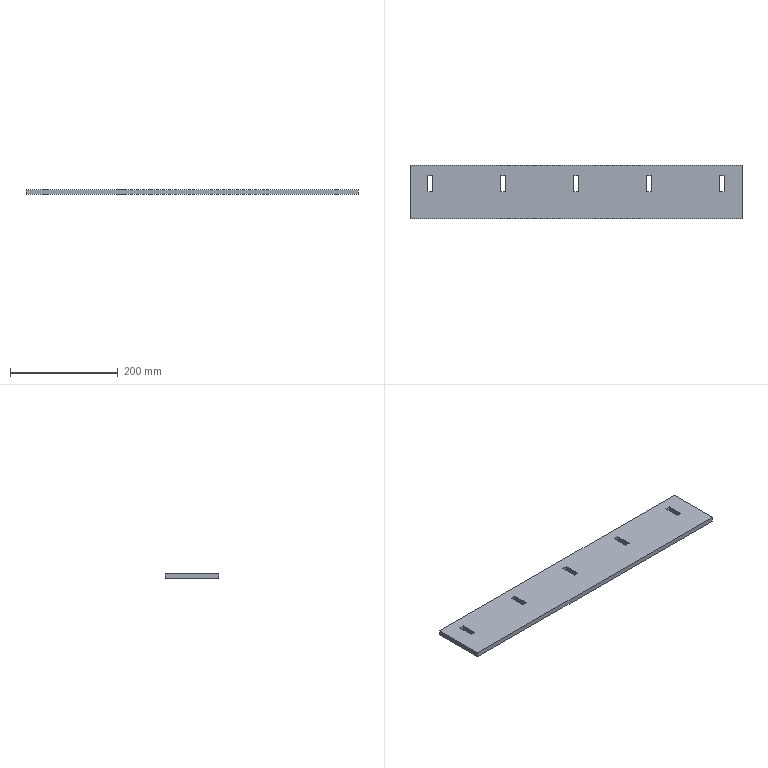Part | SolidWorks | features FlatPattern 1, SMBaseFlange 1, SheetMetal 1 | 1 solid | 26 faces | box 615 x 100 x 9 mm | volume 541350 mm3 | plane 26
STEP:
#1=CARTESIAN_POINT('',(269.54,-128.583,9.));
#2=VERTEX_POINT('',#1);
#3=CARTESIAN_POINT('',(269.54,-28.583,9.));
#4=VERTEX_POINT('',#3);
#5=CARTESIAN_POINT('',(269.54,-128.583,9.));
#6=DIRECTION('',(0.,1.,0.));
#7=VECTOR('',#6,1000.);
#8=LINE('',#5,#7);
#9=EDGE_CURVE('',#2,#4,#8,.T.);
#10=ORIENTED_EDGE('',*,*,#9,.T.);
#11=CARTESIAN_POINT('',(-345.46,-28.583,9.));
#12=VERTEX_POINT('',#11);
#13=CARTESIAN_POINT('',(269.54,-28.583,9.));
#14=DIRECTION('',(-1.,0.,0.));
#15=VECTOR('',#14,1000.);
#16=LINE('',#13,#15);
#17=EDGE_CURVE('',#4,#12,#16,.T.);
#18=ORIENTED_EDGE('',*,*,#17,.T.);
#19=CARTESIAN_POINT('',(-345.46,-128.583,9.));
#20=VERTEX_POINT('',#19);
#21=CARTESIAN_POINT('',(-345.46,-128.583,9.));
#22=DIRECTION('',(0.,-1.,0.));
#23=VECTOR('',#22,1000.);
#24=LINE('',#21,#23);
#25=EDGE_CURVE('',#12,#20,#24,.T.);
#26=ORIENTED_EDGE('',*,*,#25,.T.);
#27=CARTESIAN_POINT('',(269.54,-128.583,9.));
#28=DIRECTION('',(1.,0.,0.));
#29=VECTOR('',#28,1000.);
#30=LINE('',#27,#29);
#31=EDGE_CURVE('',#20,#2,#30,.T.);
#32=ORIENTED_EDGE('',*,*,#31,.T.);
#33=EDGE_LOOP('',(#10,#18,#26,#32));
#34=FACE_OUTER_BOUND('',#33,.T.);
#35=CARTESIAN_POINT('',(236.54,-48.583,9.));
#36=VERTEX_POINT('',#35);
#37=CARTESIAN_POINT('',(227.54,-48.583,9.));
#38=VERTEX_POINT('',#37);
#39=CARTESIAN_POINT('',(236.54,-48.583,9.));
#40=DIRECTION('',(-1.,0.,0.));
#41=VECTOR('',#40,1000.);
#42=LINE('',#39,#41);
#43=EDGE_CURVE('',#36,#38,#42,.T.);
#44=ORIENTED_EDGE('',*,*,#43,.F.);
#45=CARTESIAN_POINT('',(236.54,-78.583,9.));
#46=VERTEX_POINT('',#45);
#47=CARTESIAN_POINT('',(236.54,-48.583,9.));
#48=DIRECTION('',(0.,1.,0.));
#49=VECTOR('',#48,1000.);
#50=LINE('',#47,#49);
#51=EDGE_CURVE('',#46,#36,#50,.T.);
#52=ORIENTED_EDGE('',*,*,#51,.F.);
#53=CARTESIAN_POINT('',(227.54,-78.583,9.));
#54=VERTEX_POINT('',#53);
#55=CARTESIAN_POINT('',(236.54,-78.583,9.));
#56=DIRECTION('',(1.,0.,0.));
#57=VECTOR('',#56,1000.);
#58=LINE('',#55,#57);
#59=EDGE_CURVE('',#54,#46,#58,.T.);
#60=ORIENTED_EDGE('',*,*,#59,.F.);
#61=CARTESIAN_POINT('',(227.54,-48.583,9.));
#62=DIRECTION('',(0.,-1.,0.));
#63=VECTOR('',#62,1000.);
#64=LINE('',#61,#63);
#65=EDGE_CURVE('',#38,#54,#64,.T.);
#66=ORIENTED_EDGE('',*,*,#65,.F.);
#67=EDGE_LOOP('',(#44,#52,#60,#66));
#68=FACE_BOUND('',#67,.T.);
#69=CARTESIAN_POINT('',(92.54,-78.583,9.));
#70=VERTEX_POINT('',#69);
#71=CARTESIAN_POINT('',(101.54,-78.583,9.));
#72=VERTEX_POINT('',#71);
#73=CARTESIAN_POINT('',(92.54,-78.583,9.));
#74=DIRECTION('',(1.,0.,0.));
#75=VECTOR('',#74,1000.);
#76=LINE('',#73,#75);
#77=EDGE_CURVE('',#70,#72,#76,.T.);
#78=ORIENTED_EDGE('',*,*,#77,.F.);
#79=CARTESIAN_POINT('',(92.54,-48.583,9.));
#80=VERTEX_POINT('',#79);
#81=CARTESIAN_POINT('',(92.54,-48.583,9.));
#82=DIRECTION('',(0.,-1.,0.));
#83=VECTOR('',#82,1000.);
#84=LINE('',#81,#83);
#85=EDGE_CURVE('',#80,#70,#84,.T.);
#86=ORIENTED_EDGE('',*,*,#85,.F.);
#87=CARTESIAN_POINT('',(101.54,-48.583,9.));
#88=VERTEX_POINT('',#87);
#89=CARTESIAN_POINT('',(92.54,-48.583,9.));
#90=DIRECTION('',(-1.,0.,0.));
#91=VECTOR('',#90,1000.);
#92=LINE('',#89,#91);
#93=EDGE_CURVE('',#88,#80,#92,.T.);
#94=ORIENTED_EDGE('',*,*,#93,.F.);
#95=CARTESIAN_POINT('',(101.54,-48.583,9.));
#96=DIRECTION('',(0.,1.,0.));
#97=VECTOR('',#96,1000.);
#98=LINE('',#95,#97);
#99=EDGE_CURVE('',#72,#88,#98,.T.);
#100=ORIENTED_EDGE('',*,*,#99,.F.);
#101=EDGE_LOOP('',(#78,#86,#94,#100));
#102=FACE_BOUND('',#101,.T.);
#103=CARTESIAN_POINT('',(-42.46,-78.583,9.));
#104=VERTEX_POINT('',#103);
#105=CARTESIAN_POINT('',(-33.46,-78.583,9.));
#106=VERTEX_POINT('',#105);
#107=CARTESIAN_POINT('',(-42.46,-78.583,9.));
#108=DIRECTION('',(1.,0.,0.));
#109=VECTOR('',#108,1000.);
#110=LINE('',#107,#109);
#111=EDGE_CURVE('',#104,#106,#110,.T.);
#112=ORIENTED_EDGE('',*,*,#111,.F.);
#113=CARTESIAN_POINT('',(-42.46,-48.583,9.));
#114=VERTEX_POINT('',#113);
#115=CARTESIAN_POINT('',(-42.46,-48.583,9.));
#116=DIRECTION('',(0.,-1.,0.));
#117=VECTOR('',#116,1000.);
#118=LINE('',#115,#117);
#119=EDGE_CURVE('',#114,#104,#118,.T.);
#120=ORIENTED_EDGE('',*,*,#119,.F.);
#121=CARTESIAN_POINT('',(-33.46,-48.583,9.));
#122=VERTEX_POINT('',#121);
#123=CARTESIAN_POINT('',(-42.46,-48.583,9.));
#124=DIRECTION('',(-1.,0.,0.));
#125=VECTOR('',#124,1000.);
#126=LINE('',#123,#125);
#127=EDGE_CURVE('',#122,#114,#126,.T.);
#128=ORIENTED_EDGE('',*,*,#127,.F.);
#129=CARTESIAN_POINT('',(-33.46,-48.583,9.));
#130=DIRECTION('',(0.,1.,0.));
#131=VECTOR('',#130,1000.);
#132=LINE('',#129,#131);
#133=EDGE_CURVE('',#106,#122,#132,.T.);
#134=ORIENTED_EDGE('',*,*,#133,.F.);
#135=EDGE_LOOP('',(#112,#120,#128,#134));
#136=FACE_BOUND('',#135,.T.);
#137=CARTESIAN_POINT('',(-177.46,-78.583,9.));
#138=VERTEX_POINT('',#137);
#139=CARTESIAN_POINT('',(-168.46,-78.583,9.));
#140=VERTEX_POINT('',#139);
#141=CARTESIAN_POINT('',(-177.46,-78.583,9.));
#142=DIRECTION('',(1.,0.,0.));
#143=VECTOR('',#142,1000.);
#144=LINE('',#141,#143);
#145=EDGE_CURVE('',#138,#140,#144,.T.);
#146=ORIENTED_EDGE('',*,*,#145,.F.);
#147=CARTESIAN_POINT('',(-177.46,-48.583,9.));
#148=VERTEX_POINT('',#147);
#149=CARTESIAN_POINT('',(-177.46,-48.583,9.));
#150=DIRECTION('',(0.,-1.,0.));
#151=VECTOR('',#150,1000.);
#152=LINE('',#149,#151);
#153=EDGE_CURVE('',#148,#138,#152,.T.);
#154=ORIENTED_EDGE('',*,*,#153,.F.);
#155=CARTESIAN_POINT('',(-168.46,-48.583,9.));
#156=VERTEX_POINT('',#155);
#157=CARTESIAN_POINT('',(-177.46,-48.583,9.));
#158=DIRECTION('',(-1.,0.,0.));
#159=VECTOR('',#158,1000.);
#160=LINE('',#157,#159);
#161=EDGE_CURVE('',#156,#148,#160,.T.);
#162=ORIENTED_EDGE('',*,*,#161,.F.);
#163=CARTESIAN_POINT('',(-168.46,-48.583,9.));
#164=DIRECTION('',(0.,1.,0.));
#165=VECTOR('',#164,1000.);
#166=LINE('',#163,#165);
#167=EDGE_CURVE('',#140,#156,#166,.T.);
#168=ORIENTED_EDGE('',*,*,#167,.F.);
#169=EDGE_LOOP('',(#146,#154,#162,#168));
#170=FACE_BOUND('',#169,.T.);
#171=CARTESIAN_POINT('',(-312.46,-78.583,9.));
#172=VERTEX_POINT('',#171);
#173=CARTESIAN_POINT('',(-303.46,-78.583,9.));
#174=VERTEX_POINT('',#173);
#175=CARTESIAN_POINT('',(-312.46,-78.583,9.));
#176=DIRECTION('',(1.,0.,0.));
#177=VECTOR('',#176,1000.);
#178=LINE('',#175,#177);
#179=EDGE_CURVE('',#172,#174,#178,.T.);
#180=ORIENTED_EDGE('',*,*,#179,.F.);
#181=CARTESIAN_POINT('',(-312.46,-48.583,9.));
#182=VERTEX_POINT('',#181);
#183=CARTESIAN_POINT('',(-312.46,-48.583,9.));
#184=DIRECTION('',(0.,-1.,0.));
#185=VECTOR('',#184,1000.);
#186=LINE('',#183,#185);
#187=EDGE_CURVE('',#182,#172,#186,.T.);
#188=ORIENTED_EDGE('',*,*,#187,.F.);
#189=CARTESIAN_POINT('',(-303.46,-48.583,9.));
#190=VERTEX_POINT('',#189);
#191=CARTESIAN_POINT('',(-312.46,-48.583,9.));
#192=DIRECTION('',(-1.,0.,0.));
#193=VECTOR('',#192,1000.);
#194=LINE('',#191,#193);
#195=EDGE_CURVE('',#190,#182,#194,.T.);
#196=ORIENTED_EDGE('',*,*,#195,.F.);
#197=CARTESIAN_POINT('',(-303.46,-48.583,9.));
#198=DIRECTION('',(0.,1.,0.));
#199=VECTOR('',#198,1000.);
#200=LINE('',#197,#199);
#201=EDGE_CURVE('',#174,#190,#200,.T.);
#202=ORIENTED_EDGE('',*,*,#201,.F.);
#203=EDGE_LOOP('',(#180,#188,#196,#202));
#204=FACE_BOUND('',#203,.T.);
#205=CARTESIAN_POINT('',(0.,0.,9.));
#206=DIRECTION('',(0.,0.,1.));
#207=DIRECTION('',(1.,0.,0.));
#208=AXIS2_PLACEMENT_3D('',#205,#206,#207);
#209=PLANE('',#208);
#210=ADVANCED_FACE('',(#34,#68,#102,#136,#170,#204),#209,.T.);
#211=CARTESIAN_POINT('',(-177.46,-48.583,0.));
#212=VERTEX_POINT('',#211);
#213=CARTESIAN_POINT('',(-177.46,-78.583,0.));
#214=VERTEX_POINT('',#213);
#215=CARTESIAN_POINT('',(-177.46,-48.583,0.));
#216=DIRECTION('',(0.,-1.,0.));
#217=VECTOR('',#216,1000.);
#218=LINE('',#215,#217);
#219=EDGE_CURVE('',#212,#214,#218,.T.);
#220=ORIENTED_EDGE('',*,*,#219,.T.);
#221=CARTESIAN_POINT('',(-168.46,-78.583,0.));
#222=VERTEX_POINT('',#221);
#223=CARTESIAN_POINT('',(-177.46,-78.583,0.));
#224=DIRECTION('',(1.,0.,0.));
#225=VECTOR('',#224,1000.);
#226=LINE('',#223,#225);
#227=EDGE_CURVE('',#214,#222,#226,.T.);
#228=ORIENTED_EDGE('',*,*,#227,.T.);
#229=CARTESIAN_POINT('',(-168.46,-48.583,0.));
#230=VERTEX_POINT('',#229);
#231=CARTESIAN_POINT('',(-168.46,-48.583,0.));
#232=DIRECTION('',(0.,1.,0.));
#233=VECTOR('',#232,1000.);
#234=LINE('',#231,#233);
#235=EDGE_CURVE('',#222,#230,#234,.T.);
#236=ORIENTED_EDGE('',*,*,#235,.T.);
#237=CARTESIAN_POINT('',(-177.46,-48.583,0.));
#238=DIRECTION('',(-1.,0.,0.));
#239=VECTOR('',#238,1000.);
#240=LINE('',#237,#239);
#241=EDGE_CURVE('',#230,#212,#240,.T.);
#242=ORIENTED_EDGE('',*,*,#241,.T.);
#243=EDGE_LOOP('',(#220,#228,#236,#242));
#244=FACE_BOUND('',#243,.T.);
#245=CARTESIAN_POINT('',(92.54,-48.583,0.));
#246=VERTEX_POINT('',#245);
#247=CARTESIAN_POINT('',(92.54,-78.583,0.));
#248=VERTEX_POINT('',#247);
#249=CARTESIAN_POINT('',(92.54,-48.583,0.));
#250=DIRECTION('',(0.,-1.,0.));
#251=VECTOR('',#250,1000.);
#252=LINE('',#249,#251);
#253=EDGE_CURVE('',#246,#248,#252,.T.);
#254=ORIENTED_EDGE('',*,*,#253,.T.);
#255=CARTESIAN_POINT('',(101.54,-78.583,0.));
#256=VERTEX_POINT('',#255);
#257=CARTESIAN_POINT('',(92.54,-78.583,0.));
#258=DIRECTION('',(1.,0.,0.));
#259=VECTOR('',#258,1000.);
#260=LINE('',#257,#259);
#261=EDGE_CURVE('',#248,#256,#260,.T.);
#262=ORIENTED_EDGE('',*,*,#261,.T.);
#263=CARTESIAN_POINT('',(101.54,-48.583,0.));
#264=VERTEX_POINT('',#263);
#265=CARTESIAN_POINT('',(101.54,-48.583,0.));
#266=DIRECTION('',(0.,1.,0.));
#267=VECTOR('',#266,1000.);
#268=LINE('',#265,#267);
#269=EDGE_CURVE('',#256,#264,#268,.T.);
#270=ORIENTED_EDGE('',*,*,#269,.T.);
#271=CARTESIAN_POINT('',(92.54,-48.583,0.));
#272=DIRECTION('',(-1.,0.,0.));
#273=VECTOR('',#272,1000.);
#274=LINE('',#271,#273);
#275=EDGE_CURVE('',#264,#246,#274,.T.);
#276=ORIENTED_EDGE('',*,*,#275,.T.);
#277=EDGE_LOOP('',(#254,#262,#270,#276));
#278=FACE_BOUND('',#277,.T.);
#279=CARTESIAN_POINT('',(269.54,-128.583,0.));
#280=VERTEX_POINT('',#279);
#281=CARTESIAN_POINT('',(269.54,-28.583,0.));
#282=VERTEX_POINT('',#281);
#283=CARTESIAN_POINT('',(269.54,-128.583,0.));
#284=DIRECTION('',(0.,1.,0.));
#285=VECTOR('',#284,1000.);
#286=LINE('',#283,#285);
#287=EDGE_CURVE('',#280,#282,#286,.T.);
#288=ORIENTED_EDGE('',*,*,#287,.F.);
#289=CARTESIAN_POINT('',(-345.46,-128.583,0.));
#290=VERTEX_POINT('',#289);
#291=CARTESIAN_POINT('',(269.54,-128.583,0.));
#292=DIRECTION('',(1.,0.,0.));
#293=VECTOR('',#292,1000.);
#294=LINE('',#291,#293);
#295=EDGE_CURVE('',#290,#280,#294,.T.);
#296=ORIENTED_EDGE('',*,*,#295,.F.);
#297=CARTESIAN_POINT('',(-345.46,-28.583,0.));
#298=VERTEX_POINT('',#297);
#299=CARTESIAN_POINT('',(-345.46,-128.583,0.));
#300=DIRECTION('',(0.,-1.,0.));
#301=VECTOR('',#300,1000.);
#302=LINE('',#299,#301);
#303=EDGE_CURVE('',#298,#290,#302,.T.);
#304=ORIENTED_EDGE('',*,*,#303,.F.);
#305=CARTESIAN_POINT('',(269.54,-28.583,0.));
#306=DIRECTION('',(-1.,0.,0.));
#307=VECTOR('',#306,1000.);
#308=LINE('',#305,#307);
#309=EDGE_CURVE('',#282,#298,#308,.T.);
#310=ORIENTED_EDGE('',*,*,#309,.F.);
#311=EDGE_LOOP('',(#288,#296,#304,#310));
#312=FACE_OUTER_BOUND('',#311,.T.);
#313=CARTESIAN_POINT('',(236.54,-78.583,0.));
#314=VERTEX_POINT('',#313);
#315=CARTESIAN_POINT('',(236.54,-48.583,0.));
#316=VERTEX_POINT('',#315);
#317=CARTESIAN_POINT('',(236.54,-48.583,0.));
#318=DIRECTION('',(0.,1.,0.));
#319=VECTOR('',#318,1000.);
#320=LINE('',#317,#319);
#321=EDGE_CURVE('',#314,#316,#320,.T.);
#322=ORIENTED_EDGE('',*,*,#321,.T.);
#323=CARTESIAN_POINT('',(227.54,-48.583,0.));
#324=VERTEX_POINT('',#323);
#325=CARTESIAN_POINT('',(236.54,-48.583,0.));
#326=DIRECTION('',(-1.,0.,0.));
#327=VECTOR('',#326,1000.);
#328=LINE('',#325,#327);
#329=EDGE_CURVE('',#316,#324,#328,.T.);
#330=ORIENTED_EDGE('',*,*,#329,.T.);
#331=CARTESIAN_POINT('',(227.54,-78.583,0.));
#332=VERTEX_POINT('',#331);
#333=CARTESIAN_POINT('',(227.54,-48.583,0.));
#334=DIRECTION('',(0.,-1.,0.));
#335=VECTOR('',#334,1000.);
#336=LINE('',#333,#335);
#337=EDGE_CURVE('',#324,#332,#336,.T.);
#338=ORIENTED_EDGE('',*,*,#337,.T.);
#339=CARTESIAN_POINT('',(236.54,-78.583,0.));
#340=DIRECTION('',(1.,0.,0.));
#341=VECTOR('',#340,1000.);
#342=LINE('',#339,#341);
#343=EDGE_CURVE('',#332,#314,#342,.T.);
#344=ORIENTED_EDGE('',*,*,#343,.T.);
#345=EDGE_LOOP('',(#322,#330,#338,#344));
#346=FACE_BOUND('',#345,.T.);
#347=CARTESIAN_POINT('',(-42.46,-48.583,0.));
#348=VERTEX_POINT('',#347);
#349=CARTESIAN_POINT('',(-42.46,-78.583,0.));
#350=VERTEX_POINT('',#349);
#351=CARTESIAN_POINT('',(-42.46,-48.583,0.));
#352=DIRECTION('',(0.,-1.,0.));
#353=VECTOR('',#352,1000.);
#354=LINE('',#351,#353);
#355=EDGE_CURVE('',#348,#350,#354,.T.);
#356=ORIENTED_EDGE('',*,*,#355,.T.);
#357=CARTESIAN_POINT('',(-33.46,-78.583,0.));
#358=VERTEX_POINT('',#357);
#359=CARTESIAN_POINT('',(-42.46,-78.583,0.));
#360=DIRECTION('',(1.,0.,0.));
#361=VECTOR('',#360,1000.);
#362=LINE('',#359,#361);
#363=EDGE_CURVE('',#350,#358,#362,.T.);
#364=ORIENTED_EDGE('',*,*,#363,.T.);
#365=CARTESIAN_POINT('',(-33.46,-48.583,0.));
#366=VERTEX_POINT('',#365);
#367=CARTESIAN_POINT('',(-33.46,-48.583,0.));
#368=DIRECTION('',(0.,1.,0.));
#369=VECTOR('',#368,1000.);
#370=LINE('',#367,#369);
#371=EDGE_CURVE('',#358,#366,#370,.T.);
#372=ORIENTED_EDGE('',*,*,#371,.T.);
#373=CARTESIAN_POINT('',(-42.46,-48.583,0.));
#374=DIRECTION('',(-1.,0.,0.));
#375=VECTOR('',#374,1000.);
#376=LINE('',#373,#375);
#377=EDGE_CURVE('',#366,#348,#376,.T.);
#378=ORIENTED_EDGE('',*,*,#377,.T.);
#379=EDGE_LOOP('',(#356,#364,#372,#378));
#380=FACE_BOUND('',#379,.T.);
#381=CARTESIAN_POINT('',(-312.46,-48.583,0.));
#382=VERTEX_POINT('',#381);
#383=CARTESIAN_POINT('',(-312.46,-78.583,0.));
#384=VERTEX_POINT('',#383);
#385=CARTESIAN_POINT('',(-312.46,-48.583,0.));
#386=DIRECTION('',(0.,-1.,0.));
#387=VECTOR('',#386,1000.);
#388=LINE('',#385,#387);
#389=EDGE_CURVE('',#382,#384,#388,.T.);
#390=ORIENTED_EDGE('',*,*,#389,.T.);
#391=CARTESIAN_POINT('',(-303.46,-78.583,0.));
#392=VERTEX_POINT('',#391);
#393=CARTESIAN_POINT('',(-312.46,-78.583,0.));
#394=DIRECTION('',(1.,0.,0.));
#395=VECTOR('',#394,1000.);
#396=LINE('',#393,#395);
#397=EDGE_CURVE('',#384,#392,#396,.T.);
#398=ORIENTED_EDGE('',*,*,#397,.T.);
#399=CARTESIAN_POINT('',(-303.46,-48.583,0.));
#400=VERTEX_POINT('',#399);
#401=CARTESIAN_POINT('',(-303.46,-48.583,0.));
#402=DIRECTION('',(0.,1.,0.));
#403=VECTOR('',#402,1000.);
#404=LINE('',#401,#403);
#405=EDGE_CURVE('',#392,#400,#404,.T.);
#406=ORIENTED_EDGE('',*,*,#405,.T.);
#407=CARTESIAN_POINT('',(-312.46,-48.583,0.));
#408=DIRECTION('',(-1.,0.,0.));
#409=VECTOR('',#408,1000.);
#410=LINE('',#407,#409);
#411=EDGE_CURVE('',#400,#382,#410,.T.);
#412=ORIENTED_EDGE('',*,*,#411,.T.);
#413=EDGE_LOOP('',(#390,#398,#406,#412));
#414=FACE_BOUND('',#413,.T.);
#415=CARTESIAN_POINT('',(0.,0.,0.));
#416=DIRECTION('',(0.,0.,1.));
#417=DIRECTION('',(1.,0.,0.));
#418=AXIS2_PLACEMENT_3D('',#415,#416,#417);
#419=PLANE('',#418);
#420=ADVANCED_FACE('',(#244,#278,#312,#346,#380,#414),#419,.F.);
#421=ORIENTED_EDGE('',*,*,#287,.T.);
#422=CARTESIAN_POINT('',(269.54,-28.583,9.));
#423=DIRECTION('',(0.,0.,-1.));
#424=VECTOR('',#423,1000.);
#425=LINE('',#422,#424);
#426=EDGE_CURVE('',#4,#282,#425,.T.);
#427=ORIENTED_EDGE('',*,*,#426,.F.);
#428=ORIENTED_EDGE('',*,*,#9,.F.);
#429=CARTESIAN_POINT('',(269.54,-128.583,9.));
#430=DIRECTION('',(0.,0.,-1.));
#431=VECTOR('',#430,1000.);
#432=LINE('',#429,#431);
#433=EDGE_CURVE('',#2,#280,#432,.T.);
#434=ORIENTED_EDGE('',*,*,#433,.T.);
#435=EDGE_LOOP('',(#421,#427,#428,#434));
#436=FACE_OUTER_BOUND('',#435,.T.);
#437=CARTESIAN_POINT('',(269.54,-128.583,9.));
#438=DIRECTION('',(-1.,0.,0.));
#439=DIRECTION('',(0.,0.,1.));
#440=AXIS2_PLACEMENT_3D('',#437,#438,#439);
#441=PLANE('',#440);
#442=ADVANCED_FACE('',(#436),#441,.F.);
#443=ORIENTED_EDGE('',*,*,#309,.T.);
#444=CARTESIAN_POINT('',(-345.46,-28.583,9.));
#445=DIRECTION('',(0.,0.,-1.));
#446=VECTOR('',#445,1000.);
#447=LINE('',#444,#446);
#448=EDGE_CURVE('',#12,#298,#447,.T.);
#449=ORIENTED_EDGE('',*,*,#448,.F.);
#450=ORIENTED_EDGE('',*,*,#17,.F.);
#451=ORIENTED_EDGE('',*,*,#426,.T.);
#452=EDGE_LOOP('',(#443,#449,#450,#451));
#453=FACE_OUTER_BOUND('',#452,.T.);
#454=CARTESIAN_POINT('',(269.54,-28.583,9.));
#455=DIRECTION('',(0.,-1.,0.));
#456=DIRECTION('',(1.,0.,0.));
#457=AXIS2_PLACEMENT_3D('',#454,#455,#456);
#458=PLANE('',#457);
#459=ADVANCED_FACE('',(#453),#458,.F.);
#460=ORIENTED_EDGE('',*,*,#303,.T.);
#461=CARTESIAN_POINT('',(-345.46,-128.583,9.));
#462=DIRECTION('',(0.,0.,-1.));
#463=VECTOR('',#462,1000.);
#464=LINE('',#461,#463);
#465=EDGE_CURVE('',#20,#290,#464,.T.);
#466=ORIENTED_EDGE('',*,*,#465,.F.);
#467=ORIENTED_EDGE('',*,*,#25,.F.);
#468=ORIENTED_EDGE('',*,*,#448,.T.);
#469=EDGE_LOOP('',(#460,#466,#467,#468));
#470=FACE_OUTER_BOUND('',#469,.T.);
#471=CARTESIAN_POINT('',(-345.46,-128.583,9.));
#472=DIRECTION('',(1.,0.,0.));
#473=DIRECTION('',(0.,0.,-1.));
#474=AXIS2_PLACEMENT_3D('',#471,#472,#473);
#475=PLANE('',#474);
#476=ADVANCED_FACE('',(#470),#475,.F.);
#477=ORIENTED_EDGE('',*,*,#295,.T.);
#478=ORIENTED_EDGE('',*,*,#433,.F.);
#479=ORIENTED_EDGE('',*,*,#31,.F.);
#480=ORIENTED_EDGE('',*,*,#465,.T.);
#481=EDGE_LOOP('',(#477,#478,#479,#480));
#482=FACE_OUTER_BOUND('',#481,.T.);
#483=CARTESIAN_POINT('',(269.54,-128.583,9.));
#484=DIRECTION('',(0.,1.,0.));
#485=DIRECTION('',(-1.,0.,0.));
#486=AXIS2_PLACEMENT_3D('',#483,#484,#485);
#487=PLANE('',#486);
#488=ADVANCED_FACE('',(#482),#487,.F.);
#489=ORIENTED_EDGE('',*,*,#321,.F.);
#490=CARTESIAN_POINT('',(236.54,-78.583,9.));
#491=DIRECTION('',(0.,0.,-1.));
#492=VECTOR('',#491,1000.);
#493=LINE('',#490,#492);
#494=EDGE_CURVE('',#46,#314,#493,.T.);
#495=ORIENTED_EDGE('',*,*,#494,.F.);
#496=ORIENTED_EDGE('',*,*,#51,.T.);
#497=CARTESIAN_POINT('',(236.54,-48.583,9.));
#498=DIRECTION('',(0.,0.,-1.));
#499=VECTOR('',#498,1000.);
#500=LINE('',#497,#499);
#501=EDGE_CURVE('',#36,#316,#500,.T.);
#502=ORIENTED_EDGE('',*,*,#501,.T.);
#503=EDGE_LOOP('',(#489,#495,#496,#502));
#504=FACE_OUTER_BOUND('',#503,.T.);
#505=CARTESIAN_POINT('',(236.54,-48.583,9.));
#506=DIRECTION('',(-1.,0.,0.));
#507=DIRECTION('',(0.,0.,1.));
#508=AXIS2_PLACEMENT_3D('',#505,#506,#507);
#509=PLANE('',#508);
#510=ADVANCED_FACE('',(#504),#509,.T.);
#511=ORIENTED_EDGE('',*,*,#329,.F.);
#512=ORIENTED_EDGE('',*,*,#501,.F.);
#513=ORIENTED_EDGE('',*,*,#43,.T.);
#514=CARTESIAN_POINT('',(227.54,-48.583,9.));
#515=DIRECTION('',(0.,0.,-1.));
#516=VECTOR('',#515,1000.);
#517=LINE('',#514,#516);
#518=EDGE_CURVE('',#38,#324,#517,.T.);
#519=ORIENTED_EDGE('',*,*,#518,.T.);
#520=EDGE_LOOP('',(#511,#512,#513,#519));
#521=FACE_OUTER_BOUND('',#520,.T.);
#522=CARTESIAN_POINT('',(236.54,-48.583,9.));
#523=DIRECTION('',(0.,-1.,0.));
#524=DIRECTION('',(0.,0.,-1.));
#525=AXIS2_PLACEMENT_3D('',#522,#523,#524);
#526=PLANE('',#525);
#527=ADVANCED_FACE('',(#521),#526,.T.);
#528=ORIENTED_EDGE('',*,*,#337,.F.);
#529=ORIENTED_EDGE('',*,*,#518,.F.);
#530=ORIENTED_EDGE('',*,*,#65,.T.);
#531=CARTESIAN_POINT('',(227.54,-78.583,9.));
#532=DIRECTION('',(0.,0.,-1.));
#533=VECTOR('',#532,1000.);
#534=LINE('',#531,#533);
#535=EDGE_CURVE('',#54,#332,#534,.T.);
#536=ORIENTED_EDGE('',*,*,#535,.T.);
#537=EDGE_LOOP('',(#528,#529,#530,#536));
#538=FACE_OUTER_BOUND('',#537,.T.);
#539=CARTESIAN_POINT('',(227.54,-48.583,9.));
#540=DIRECTION('',(1.,0.,0.));
#541=DIRECTION('',(0.,0.,-1.));
#542=AXIS2_PLACEMENT_3D('',#539,#540,#541);
#543=PLANE('',#542);
#544=ADVANCED_FACE('',(#538),#543,.T.);
#545=ORIENTED_EDGE('',*,*,#343,.F.);
#546=ORIENTED_EDGE('',*,*,#535,.F.);
#547=ORIENTED_EDGE('',*,*,#59,.T.);
#548=ORIENTED_EDGE('',*,*,#494,.T.);
#549=EDGE_LOOP('',(#545,#546,#547,#548));
#550=FACE_OUTER_BOUND('',#549,.T.);
#551=CARTESIAN_POINT('',(236.54,-78.583,9.));
#552=DIRECTION('',(0.,1.,0.));
#553=DIRECTION('',(0.,0.,1.));
#554=AXIS2_PLACEMENT_3D('',#551,#552,#553);
#555=PLANE('',#554);
#556=ADVANCED_FACE('',(#550),#555,.T.);
#557=ORIENTED_EDGE('',*,*,#253,.F.);
#558=CARTESIAN_POINT('',(92.54,-48.583,9.));
#559=DIRECTION('',(0.,0.,-1.));
#560=VECTOR('',#559,1000.);
#561=LINE('',#558,#560);
#562=EDGE_CURVE('',#80,#246,#561,.T.);
#563=ORIENTED_EDGE('',*,*,#562,.F.);
#564=ORIENTED_EDGE('',*,*,#85,.T.);
#565=CARTESIAN_POINT('',(92.54,-78.583,9.));
#566=DIRECTION('',(0.,0.,-1.));
#567=VECTOR('',#566,1000.);
#568=LINE('',#565,#567);
#569=EDGE_CURVE('',#70,#248,#568,.T.);
#570=ORIENTED_EDGE('',*,*,#569,.T.);
#571=EDGE_LOOP('',(#557,#563,#564,#570));
#572=FACE_OUTER_BOUND('',#571,.T.);
#573=CARTESIAN_POINT('',(92.54,-48.583,9.));
#574=DIRECTION('',(1.,0.,0.));
#575=DIRECTION('',(0.,0.,-1.));
#576=AXIS2_PLACEMENT_3D('',#573,#574,#575);
#577=PLANE('',#576);
#578=ADVANCED_FACE('',(#572),#577,.T.);
#579=ORIENTED_EDGE('',*,*,#261,.F.);
#580=ORIENTED_EDGE('',*,*,#569,.F.);
#581=ORIENTED_EDGE('',*,*,#77,.T.);
#582=CARTESIAN_POINT('',(101.54,-78.583,9.));
#583=DIRECTION('',(0.,0.,-1.));
#584=VECTOR('',#583,1000.);
#585=LINE('',#582,#584);
#586=EDGE_CURVE('',#72,#256,#585,.T.);
#587=ORIENTED_EDGE('',*,*,#586,.T.);
#588=EDGE_LOOP('',(#579,#580,#581,#587));
#589=FACE_OUTER_BOUND('',#588,.T.);
#590=CARTESIAN_POINT('',(92.54,-78.583,9.));
#591=DIRECTION('',(0.,1.,0.));
#592=DIRECTION('',(0.,0.,1.));
#593=AXIS2_PLACEMENT_3D('',#590,#591,#592);
#594=PLANE('',#593);
#595=ADVANCED_FACE('',(#589),#594,.T.);
#596=ORIENTED_EDGE('',*,*,#269,.F.);
#597=ORIENTED_EDGE('',*,*,#586,.F.);
#598=ORIENTED_EDGE('',*,*,#99,.T.);
#599=CARTESIAN_POINT('',(101.54,-48.583,9.));
#600=DIRECTION('',(0.,0.,-1.));
#601=VECTOR('',#600,1000.);
#602=LINE('',#599,#601);
#603=EDGE_CURVE('',#88,#264,#602,.T.);
#604=ORIENTED_EDGE('',*,*,#603,.T.);
#605=EDGE_LOOP('',(#596,#597,#598,#604));
#606=FACE_OUTER_BOUND('',#605,.T.);
#607=CARTESIAN_POINT('',(101.54,-48.583,9.));
#608=DIRECTION('',(-1.,0.,0.));
#609=DIRECTION('',(0.,0.,1.));
#610=AXIS2_PLACEMENT_3D('',#607,#608,#609);
#611=PLANE('',#610);
#612=ADVANCED_FACE('',(#606),#611,.T.);
#613=ORIENTED_EDGE('',*,*,#275,.F.);
#614=ORIENTED_EDGE('',*,*,#603,.F.);
#615=ORIENTED_EDGE('',*,*,#93,.T.);
#616=ORIENTED_EDGE('',*,*,#562,.T.);
#617=EDGE_LOOP('',(#613,#614,#615,#616));
#618=FACE_OUTER_BOUND('',#617,.T.);
#619=CARTESIAN_POINT('',(92.54,-48.583,9.));
#620=DIRECTION('',(0.,-1.,0.));
#621=DIRECTION('',(0.,0.,-1.));
#622=AXIS2_PLACEMENT_3D('',#619,#620,#621);
#623=PLANE('',#622);
#624=ADVANCED_FACE('',(#618),#623,.T.);
#625=ORIENTED_EDGE('',*,*,#355,.F.);
#626=CARTESIAN_POINT('',(-42.46,-48.583,9.));
#627=DIRECTION('',(0.,0.,-1.));
#628=VECTOR('',#627,1000.);
#629=LINE('',#626,#628);
#630=EDGE_CURVE('',#114,#348,#629,.T.);
#631=ORIENTED_EDGE('',*,*,#630,.F.);
#632=ORIENTED_EDGE('',*,*,#119,.T.);
#633=CARTESIAN_POINT('',(-42.46,-78.583,9.));
#634=DIRECTION('',(0.,0.,-1.));
#635=VECTOR('',#634,1000.);
#636=LINE('',#633,#635);
#637=EDGE_CURVE('',#104,#350,#636,.T.);
#638=ORIENTED_EDGE('',*,*,#637,.T.);
#639=EDGE_LOOP('',(#625,#631,#632,#638));
#640=FACE_OUTER_BOUND('',#639,.T.);
#641=CARTESIAN_POINT('',(-42.46,-48.583,9.));
#642=DIRECTION('',(1.,0.,0.));
#643=DIRECTION('',(0.,0.,-1.));
#644=AXIS2_PLACEMENT_3D('',#641,#642,#643);
#645=PLANE('',#644);
#646=ADVANCED_FACE('',(#640),#645,.T.);
#647=ORIENTED_EDGE('',*,*,#363,.F.);
#648=ORIENTED_EDGE('',*,*,#637,.F.);
#649=ORIENTED_EDGE('',*,*,#111,.T.);
#650=CARTESIAN_POINT('',(-33.46,-78.583,9.));
#651=DIRECTION('',(0.,0.,-1.));
#652=VECTOR('',#651,1000.);
#653=LINE('',#650,#652);
#654=EDGE_CURVE('',#106,#358,#653,.T.);
#655=ORIENTED_EDGE('',*,*,#654,.T.);
#656=EDGE_LOOP('',(#647,#648,#649,#655));
#657=FACE_OUTER_BOUND('',#656,.T.);
#658=CARTESIAN_POINT('',(-42.46,-78.583,9.));
#659=DIRECTION('',(0.,1.,0.));
#660=DIRECTION('',(0.,0.,1.));
#661=AXIS2_PLACEMENT_3D('',#658,#659,#660);
#662=PLANE('',#661);
#663=ADVANCED_FACE('',(#657),#662,.T.);
#664=ORIENTED_EDGE('',*,*,#371,.F.);
#665=ORIENTED_EDGE('',*,*,#654,.F.);
#666=ORIENTED_EDGE('',*,*,#133,.T.);
#667=CARTESIAN_POINT('',(-33.46,-48.583,9.));
#668=DIRECTION('',(0.,0.,-1.));
#669=VECTOR('',#668,1000.);
#670=LINE('',#667,#669);
#671=EDGE_CURVE('',#122,#366,#670,.T.);
#672=ORIENTED_EDGE('',*,*,#671,.T.);
#673=EDGE_LOOP('',(#664,#665,#666,#672));
#674=FACE_OUTER_BOUND('',#673,.T.);
#675=CARTESIAN_POINT('',(-33.46,-48.583,9.));
#676=DIRECTION('',(-1.,0.,0.));
#677=DIRECTION('',(0.,0.,1.));
#678=AXIS2_PLACEMENT_3D('',#675,#676,#677);
#679=PLANE('',#678);
#680=ADVANCED_FACE('',(#674),#679,.T.);
#681=ORIENTED_EDGE('',*,*,#377,.F.);
#682=ORIENTED_EDGE('',*,*,#671,.F.);
#683=ORIENTED_EDGE('',*,*,#127,.T.);
#684=ORIENTED_EDGE('',*,*,#630,.T.);
#685=EDGE_LOOP('',(#681,#682,#683,#684));
#686=FACE_OUTER_BOUND('',#685,.T.);
#687=CARTESIAN_POINT('',(-42.46,-48.583,9.));
#688=DIRECTION('',(0.,-1.,0.));
#689=DIRECTION('',(0.,0.,-1.));
#690=AXIS2_PLACEMENT_3D('',#687,#688,#689);
#691=PLANE('',#690);
#692=ADVANCED_FACE('',(#686),#691,.T.);
#693=ORIENTED_EDGE('',*,*,#219,.F.);
#694=CARTESIAN_POINT('',(-177.46,-48.583,9.));
#695=DIRECTION('',(0.,0.,-1.));
#696=VECTOR('',#695,1000.);
#697=LINE('',#694,#696);
#698=EDGE_CURVE('',#148,#212,#697,.T.);
#699=ORIENTED_EDGE('',*,*,#698,.F.);
#700=ORIENTED_EDGE('',*,*,#153,.T.);
#701=CARTESIAN_POINT('',(-177.46,-78.583,9.));
#702=DIRECTION('',(0.,0.,-1.));
#703=VECTOR('',#702,1000.);
#704=LINE('',#701,#703);
#705=EDGE_CURVE('',#138,#214,#704,.T.);
#706=ORIENTED_EDGE('',*,*,#705,.T.);
#707=EDGE_LOOP('',(#693,#699,#700,#706));
#708=FACE_OUTER_BOUND('',#707,.T.);
#709=CARTESIAN_POINT('',(-177.46,-48.583,9.));
#710=DIRECTION('',(1.,0.,0.));
#711=DIRECTION('',(0.,0.,-1.));
#712=AXIS2_PLACEMENT_3D('',#709,#710,#711);
#713=PLANE('',#712);
#714=ADVANCED_FACE('',(#708),#713,.T.);
#715=ORIENTED_EDGE('',*,*,#227,.F.);
#716=ORIENTED_EDGE('',*,*,#705,.F.);
#717=ORIENTED_EDGE('',*,*,#145,.T.);
#718=CARTESIAN_POINT('',(-168.46,-78.583,9.));
#719=DIRECTION('',(0.,0.,-1.));
#720=VECTOR('',#719,1000.);
#721=LINE('',#718,#720);
#722=EDGE_CURVE('',#140,#222,#721,.T.);
#723=ORIENTED_EDGE('',*,*,#722,.T.);
#724=EDGE_LOOP('',(#715,#716,#717,#723));
#725=FACE_OUTER_BOUND('',#724,.T.);
#726=CARTESIAN_POINT('',(-177.46,-78.583,9.));
#727=DIRECTION('',(0.,1.,0.));
#728=DIRECTION('',(0.,0.,1.));
#729=AXIS2_PLACEMENT_3D('',#726,#727,#728);
#730=PLANE('',#729);
#731=ADVANCED_FACE('',(#725),#730,.T.);
#732=ORIENTED_EDGE('',*,*,#235,.F.);
#733=ORIENTED_EDGE('',*,*,#722,.F.);
#734=ORIENTED_EDGE('',*,*,#167,.T.);
#735=CARTESIAN_POINT('',(-168.46,-48.583,9.));
#736=DIRECTION('',(0.,0.,-1.));
#737=VECTOR('',#736,1000.);
#738=LINE('',#735,#737);
#739=EDGE_CURVE('',#156,#230,#738,.T.);
#740=ORIENTED_EDGE('',*,*,#739,.T.);
#741=EDGE_LOOP('',(#732,#733,#734,#740));
#742=FACE_OUTER_BOUND('',#741,.T.);
#743=CARTESIAN_POINT('',(-168.46,-48.583,9.));
#744=DIRECTION('',(-1.,0.,0.));
#745=DIRECTION('',(0.,0.,1.));
#746=AXIS2_PLACEMENT_3D('',#743,#744,#745);
#747=PLANE('',#746);
#748=ADVANCED_FACE('',(#742),#747,.T.);
#749=ORIENTED_EDGE('',*,*,#241,.F.);
#750=ORIENTED_EDGE('',*,*,#739,.F.);
#751=ORIENTED_EDGE('',*,*,#161,.T.);
#752=ORIENTED_EDGE('',*,*,#698,.T.);
#753=EDGE_LOOP('',(#749,#750,#751,#752));
#754=FACE_OUTER_BOUND('',#753,.T.);
#755=CARTESIAN_POINT('',(-177.46,-48.583,9.));
#756=DIRECTION('',(0.,-1.,0.));
#757=DIRECTION('',(0.,0.,-1.));
#758=AXIS2_PLACEMENT_3D('',#755,#756,#757);
#759=PLANE('',#758);
#760=ADVANCED_FACE('',(#754),#759,.T.);
#761=ORIENTED_EDGE('',*,*,#389,.F.);
#762=CARTESIAN_POINT('',(-312.46,-48.583,9.));
#763=DIRECTION('',(0.,0.,-1.));
#764=VECTOR('',#763,1000.);
#765=LINE('',#762,#764);
#766=EDGE_CURVE('',#182,#382,#765,.T.);
#767=ORIENTED_EDGE('',*,*,#766,.F.);
#768=ORIENTED_EDGE('',*,*,#187,.T.);
#769=CARTESIAN_POINT('',(-312.46,-78.583,9.));
#770=DIRECTION('',(0.,0.,-1.));
#771=VECTOR('',#770,1000.);
#772=LINE('',#769,#771);
#773=EDGE_CURVE('',#172,#384,#772,.T.);
#774=ORIENTED_EDGE('',*,*,#773,.T.);
#775=EDGE_LOOP('',(#761,#767,#768,#774));
#776=FACE_OUTER_BOUND('',#775,.T.);
#777=CARTESIAN_POINT('',(-312.46,-48.583,9.));
#778=DIRECTION('',(1.,0.,0.));
#779=DIRECTION('',(0.,0.,-1.));
#780=AXIS2_PLACEMENT_3D('',#777,#778,#779);
#781=PLANE('',#780);
#782=ADVANCED_FACE('',(#776),#781,.T.);
#783=ORIENTED_EDGE('',*,*,#397,.F.);
#784=ORIENTED_EDGE('',*,*,#773,.F.);
#785=ORIENTED_EDGE('',*,*,#179,.T.);
#786=CARTESIAN_POINT('',(-303.46,-78.583,9.));
#787=DIRECTION('',(0.,0.,-1.));
#788=VECTOR('',#787,1000.);
#789=LINE('',#786,#788);
#790=EDGE_CURVE('',#174,#392,#789,.T.);
#791=ORIENTED_EDGE('',*,*,#790,.T.);
#792=EDGE_LOOP('',(#783,#784,#785,#791));
#793=FACE_OUTER_BOUND('',#792,.T.);
#794=CARTESIAN_POINT('',(-312.46,-78.583,9.));
#795=DIRECTION('',(0.,1.,0.));
#796=DIRECTION('',(0.,0.,1.));
#797=AXIS2_PLACEMENT_3D('',#794,#795,#796);
#798=PLANE('',#797);
#799=ADVANCED_FACE('',(#793),#798,.T.);
#800=ORIENTED_EDGE('',*,*,#405,.F.);
#801=ORIENTED_EDGE('',*,*,#790,.F.);
#802=ORIENTED_EDGE('',*,*,#201,.T.);
#803=CARTESIAN_POINT('',(-303.46,-48.583,9.));
#804=DIRECTION('',(0.,0.,-1.));
#805=VECTOR('',#804,1000.);
#806=LINE('',#803,#805);
#807=EDGE_CURVE('',#190,#400,#806,.T.);
#808=ORIENTED_EDGE('',*,*,#807,.T.);
#809=EDGE_LOOP('',(#800,#801,#802,#808));
#810=FACE_OUTER_BOUND('',#809,.T.);
#811=CARTESIAN_POINT('',(-303.46,-48.583,9.));
#812=DIRECTION('',(-1.,0.,0.));
#813=DIRECTION('',(0.,0.,1.));
#814=AXIS2_PLACEMENT_3D('',#811,#812,#813);
#815=PLANE('',#814);
#816=ADVANCED_FACE('',(#810),#815,.T.);
#817=ORIENTED_EDGE('',*,*,#411,.F.);
#818=ORIENTED_EDGE('',*,*,#807,.F.);
#819=ORIENTED_EDGE('',*,*,#195,.T.);
#820=ORIENTED_EDGE('',*,*,#766,.T.);
#821=EDGE_LOOP('',(#817,#818,#819,#820));
#822=FACE_OUTER_BOUND('',#821,.T.);
#823=CARTESIAN_POINT('',(-312.46,-48.583,9.));
#824=DIRECTION('',(0.,-1.,0.));
#825=DIRECTION('',(0.,0.,-1.));
#826=AXIS2_PLACEMENT_3D('',#823,#824,#825);
#827=PLANE('',#826);
#828=ADVANCED_FACE('',(#822),#827,.T.);
#829=CLOSED_SHELL('',(#210,#420,#442,#459,#476,#488,#510,#527,#544,#556,#578,#595,#612,#624,#646,#663,#680,#692,#714,#731,#748,#760,#782,#799,#816,#828));
#830=MANIFOLD_SOLID_BREP('',#829);
#831=CARTESIAN_POINT('',(0.,0.,0.));
#832=DIRECTION('',(0.,0.,1.));
#833=DIRECTION('',(1.,0.,0.));
#834=AXIS2_PLACEMENT_3D('',#831,#832,#833);
#835=(LENGTH_UNIT()NAMED_UNIT(*)SI_UNIT(.MILLI.,.METRE.));
#836=UNCERTAINTY_MEASURE_WITH_UNIT(LENGTH_MEASURE(0.00001),#835,'','');
#837=(NAMED_UNIT(*)PLANE_ANGLE_UNIT()SI_UNIT($,.RADIAN.));
#838=(NAMED_UNIT(*)SI_UNIT($,.STERADIAN.)SOLID_ANGLE_UNIT());
#839=(GEOMETRIC_REPRESENTATION_CONTEXT(3)GLOBAL_UNCERTAINTY_ASSIGNED_CONTEXT((#836))GLOBAL_UNIT_ASSIGNED_CONTEXT((#835,#837,#838))REPRESENTATION_CONTEXT('',''));
#840=ADVANCED_BREP_SHAPE_REPRESENTATION('',(#830,#834),#839);